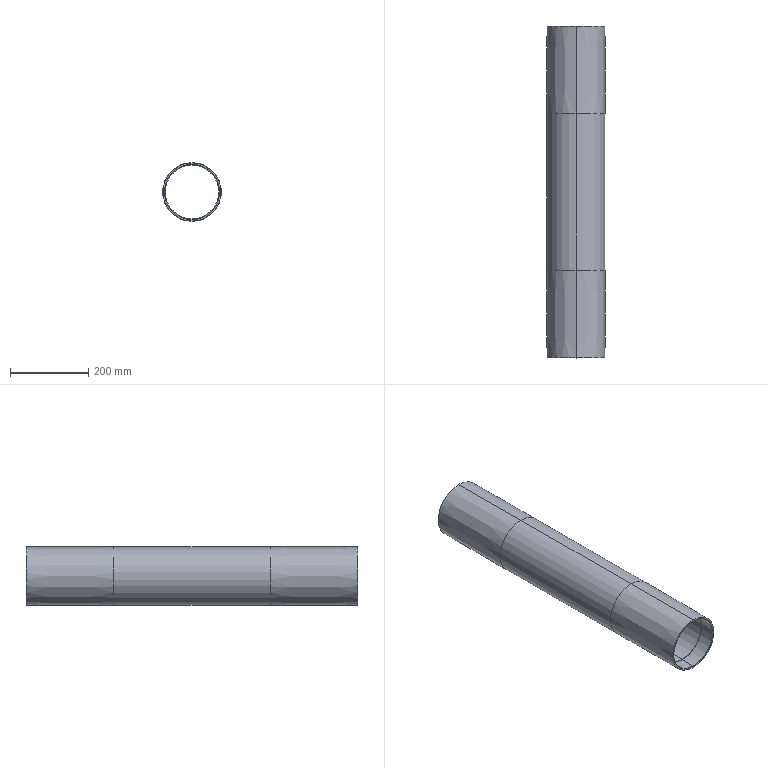Part | SolidWorks | features ICE 3, Chamfer 1, Revolution 1 | 1 solid | 20 faces | box 150 x 850 x 150 mm | volume 2218913 mm3 | cone 8 | cylinder 8 | plane 4 | commonest cylinder face diameters 140 x4 138 x2 150 x2
STEP:
#1=CARTESIAN_POINT('',(74.5,1.,70.));
#2=VERTEX_POINT('',#1);
#3=CARTESIAN_POINT('',(74.5,1.,-70.));
#4=VERTEX_POINT('',#3);
#5=CARTESIAN_POINT('',(74.5,1.,0.));
#6=DIRECTION('',(0.,-1.,0.));
#7=DIRECTION('',(0.,0.,-1.));
#8=AXIS2_PLACEMENT_3D('',#5,#6,#7);
#9=CIRCLE('',#8,70.);
#10=EDGE_CURVE('',#2,#4,#9,.T.);
#11=ORIENTED_EDGE('',*,*,#10,.F.);
#12=CARTESIAN_POINT('',(74.5,0.,71.));
#13=VERTEX_POINT('',#12);
#14=CARTESIAN_POINT('',(74.5,1.,70.));
#15=DIRECTION('',(0.,-0.7071,0.7071));
#16=VECTOR('',#15,1000.);
#17=LINE('',#14,#16);
#18=EDGE_CURVE('',#2,#13,#17,.T.);
#19=ORIENTED_EDGE('',*,*,#18,.T.);
#20=CARTESIAN_POINT('',(74.5,0.,-71.));
#21=VERTEX_POINT('',#20);
#22=CARTESIAN_POINT('',(74.5,0.,0.));
#23=DIRECTION('',(0.,1.,0.));
#24=DIRECTION('',(0.,0.,-1.));
#25=AXIS2_PLACEMENT_3D('',#22,#23,#24);
#26=CIRCLE('',#25,71.);
#27=EDGE_CURVE('',#21,#13,#26,.T.);
#28=ORIENTED_EDGE('',*,*,#27,.F.);
#29=CARTESIAN_POINT('',(74.5,1.,-70.));
#30=DIRECTION('',(0.,-0.7071,-0.7071));
#31=VECTOR('',#30,1000.);
#32=LINE('',#29,#31);
#33=EDGE_CURVE('',#4,#21,#32,.T.);
#34=ORIENTED_EDGE('',*,*,#33,.F.);
#35=EDGE_LOOP('',(#11,#19,#28,#34));
#36=FACE_OUTER_BOUND('',#35,.T.);
#37=CARTESIAN_POINT('',(74.5,1.,0.));
#38=DIRECTION('',(0.,-1.,0.));
#39=DIRECTION('',(0.,0.,-1.));
#40=AXIS2_PLACEMENT_3D('',#37,#38,#39);
#41=CONICAL_SURFACE('',#40,70.,0.7854);
#42=ADVANCED_FACE('',(#36),#41,.F.);
#43=CARTESIAN_POINT('',(74.5,849.,-70.));
#44=VERTEX_POINT('',#43);
#45=CARTESIAN_POINT('',(74.5,849.,70.));
#46=VERTEX_POINT('',#45);
#47=CARTESIAN_POINT('',(74.5,849.,0.));
#48=DIRECTION('',(0.,1.,0.));
#49=DIRECTION('',(0.,0.,1.));
#50=AXIS2_PLACEMENT_3D('',#47,#48,#49);
#51=CIRCLE('',#50,70.);
#52=EDGE_CURVE('',#44,#46,#51,.T.);
#53=ORIENTED_EDGE('',*,*,#52,.F.);
#54=CARTESIAN_POINT('',(74.5,850.,-71.));
#55=VERTEX_POINT('',#54);
#56=CARTESIAN_POINT('',(74.5,849.,-70.));
#57=DIRECTION('',(0.,0.7071,-0.7071));
#58=VECTOR('',#57,1000.);
#59=LINE('',#56,#58);
#60=EDGE_CURVE('',#44,#55,#59,.T.);
#61=ORIENTED_EDGE('',*,*,#60,.T.);
#62=CARTESIAN_POINT('',(74.5,850.,71.));
#63=VERTEX_POINT('',#62);
#64=CARTESIAN_POINT('',(74.5,850.,0.));
#65=DIRECTION('',(0.,-1.,0.));
#66=DIRECTION('',(0.,0.,1.));
#67=AXIS2_PLACEMENT_3D('',#64,#65,#66);
#68=CIRCLE('',#67,71.);
#69=EDGE_CURVE('',#63,#55,#68,.T.);
#70=ORIENTED_EDGE('',*,*,#69,.F.);
#71=CARTESIAN_POINT('',(74.5,849.,70.));
#72=DIRECTION('',(0.,0.7071,0.7071));
#73=VECTOR('',#72,1000.);
#74=LINE('',#71,#73);
#75=EDGE_CURVE('',#46,#63,#74,.T.);
#76=ORIENTED_EDGE('',*,*,#75,.F.);
#77=EDGE_LOOP('',(#53,#61,#70,#76));
#78=FACE_OUTER_BOUND('',#77,.T.);
#79=CARTESIAN_POINT('',(74.5,849.,0.));
#80=DIRECTION('',(0.,1.,0.));
#81=DIRECTION('',(0.,0.,1.));
#82=AXIS2_PLACEMENT_3D('',#79,#80,#81);
#83=CONICAL_SURFACE('',#82,70.,0.7854);
#84=ADVANCED_FACE('',(#78),#83,.F.);
#85=CARTESIAN_POINT('',(74.5,810.,-69.));
#86=VERTEX_POINT('',#85);
#87=CARTESIAN_POINT('',(74.5,810.,69.));
#88=VERTEX_POINT('',#87);
#89=CARTESIAN_POINT('',(74.5,810.,0.));
#90=DIRECTION('',(0.,1.,0.));
#91=DIRECTION('',(0.,0.,1.));
#92=AXIS2_PLACEMENT_3D('',#89,#90,#91);
#93=CIRCLE('',#92,69.);
#94=EDGE_CURVE('',#86,#88,#93,.T.);
#95=ORIENTED_EDGE('',*,*,#94,.T.);
#96=CARTESIAN_POINT('',(74.5,40.,69.));
#97=VERTEX_POINT('',#96);
#98=CARTESIAN_POINT('',(74.5,883.,69.));
#99=DIRECTION('',(0.,-1.,0.));
#100=VECTOR('',#99,1000.);
#101=LINE('',#98,#100);
#102=EDGE_CURVE('',#88,#97,#101,.T.);
#103=ORIENTED_EDGE('',*,*,#102,.T.);
#104=CARTESIAN_POINT('',(74.5,40.,-69.));
#105=VERTEX_POINT('',#104);
#106=CARTESIAN_POINT('',(74.5,40.,0.));
#107=DIRECTION('',(0.,-1.,0.));
#108=DIRECTION('',(0.,0.,-1.));
#109=AXIS2_PLACEMENT_3D('',#106,#107,#108);
#110=CIRCLE('',#109,69.);
#111=EDGE_CURVE('',#97,#105,#110,.T.);
#112=ORIENTED_EDGE('',*,*,#111,.T.);
#113=CARTESIAN_POINT('',(74.5,883.,-69.));
#114=DIRECTION('',(0.,-1.,0.));
#115=VECTOR('',#114,1000.);
#116=LINE('',#113,#115);
#117=EDGE_CURVE('',#86,#105,#116,.T.);
#118=ORIENTED_EDGE('',*,*,#117,.F.);
#119=EDGE_LOOP('',(#95,#103,#112,#118));
#120=FACE_OUTER_BOUND('',#119,.T.);
#121=CARTESIAN_POINT('',(74.5,883.,0.));
#122=DIRECTION('',(0.,-1.,0.));
#123=DIRECTION('',(0.,0.,-1.));
#124=AXIS2_PLACEMENT_3D('',#121,#122,#123);
#125=CYLINDRICAL_SURFACE('',#124,69.);
#126=ADVANCED_FACE('',(#120),#125,.F.);
#127=CARTESIAN_POINT('',(74.5,40.,70.));
#128=VERTEX_POINT('',#127);
#129=CARTESIAN_POINT('',(74.5,40.,-70.));
#130=VERTEX_POINT('',#129);
#131=CARTESIAN_POINT('',(74.5,40.,0.));
#132=DIRECTION('',(0.,-1.,0.));
#133=DIRECTION('',(0.,0.,-1.));
#134=AXIS2_PLACEMENT_3D('',#131,#132,#133);
#135=CIRCLE('',#134,70.);
#136=EDGE_CURVE('',#128,#130,#135,.T.);
#137=ORIENTED_EDGE('',*,*,#136,.F.);
#138=CARTESIAN_POINT('',(74.5,40.,70.));
#139=DIRECTION('',(0.,-1.,0.));
#140=VECTOR('',#139,1000.);
#141=LINE('',#138,#140);
#142=EDGE_CURVE('',#128,#2,#141,.T.);
#143=ORIENTED_EDGE('',*,*,#142,.T.);
#144=ORIENTED_EDGE('',*,*,#10,.T.);
#145=CARTESIAN_POINT('',(74.5,40.,-70.));
#146=DIRECTION('',(0.,-1.,0.));
#147=VECTOR('',#146,1000.);
#148=LINE('',#145,#147);
#149=EDGE_CURVE('',#130,#4,#148,.T.);
#150=ORIENTED_EDGE('',*,*,#149,.F.);
#151=EDGE_LOOP('',(#137,#143,#144,#150));
#152=FACE_OUTER_BOUND('',#151,.T.);
#153=CARTESIAN_POINT('',(74.5,40.,0.));
#154=DIRECTION('',(0.,-1.,0.));
#155=DIRECTION('',(0.,0.,-1.));
#156=AXIS2_PLACEMENT_3D('',#153,#154,#155);
#157=CYLINDRICAL_SURFACE('',#156,70.);
#158=ADVANCED_FACE('',(#152),#157,.F.);
#159=CARTESIAN_POINT('',(74.5,810.,-70.));
#160=VERTEX_POINT('',#159);
#161=CARTESIAN_POINT('',(74.5,810.,70.));
#162=VERTEX_POINT('',#161);
#163=CARTESIAN_POINT('',(74.5,810.,0.));
#164=DIRECTION('',(0.,1.,0.));
#165=DIRECTION('',(0.,0.,1.));
#166=AXIS2_PLACEMENT_3D('',#163,#164,#165);
#167=CIRCLE('',#166,70.);
#168=EDGE_CURVE('',#160,#162,#167,.T.);
#169=ORIENTED_EDGE('',*,*,#168,.F.);
#170=CARTESIAN_POINT('',(74.5,810.,-70.));
#171=DIRECTION('',(0.,1.,0.));
#172=VECTOR('',#171,1000.);
#173=LINE('',#170,#172);
#174=EDGE_CURVE('',#160,#44,#173,.T.);
#175=ORIENTED_EDGE('',*,*,#174,.T.);
#176=ORIENTED_EDGE('',*,*,#52,.T.);
#177=CARTESIAN_POINT('',(74.5,810.,70.));
#178=DIRECTION('',(0.,1.,0.));
#179=VECTOR('',#178,1000.);
#180=LINE('',#177,#179);
#181=EDGE_CURVE('',#162,#46,#180,.T.);
#182=ORIENTED_EDGE('',*,*,#181,.F.);
#183=EDGE_LOOP('',(#169,#175,#176,#182));
#184=FACE_OUTER_BOUND('',#183,.T.);
#185=CARTESIAN_POINT('',(74.5,810.,0.));
#186=DIRECTION('',(0.,1.,0.));
#187=DIRECTION('',(0.,0.,1.));
#188=AXIS2_PLACEMENT_3D('',#185,#186,#187);
#189=CYLINDRICAL_SURFACE('',#188,70.);
#190=ADVANCED_FACE('',(#184),#189,.F.);
#191=CARTESIAN_POINT('',(74.5,0.,74.5));
#192=VERTEX_POINT('',#191);
#193=CARTESIAN_POINT('',(74.5,0.,-74.5));
#194=VERTEX_POINT('',#193);
#195=CARTESIAN_POINT('',(74.5,0.,0.));
#196=DIRECTION('',(0.,1.,0.));
#197=DIRECTION('',(0.,0.,1.));
#198=AXIS2_PLACEMENT_3D('',#195,#196,#197);
#199=CIRCLE('',#198,74.5);
#200=EDGE_CURVE('',#192,#194,#199,.T.);
#201=ORIENTED_EDGE('',*,*,#200,.T.);
#202=CARTESIAN_POINT('',(74.5,225.,-75.));
#203=VERTEX_POINT('',#202);
#204=CARTESIAN_POINT('',(74.5,225.,-75.));
#205=DIRECTION('',(0.,1.,-0.002222));
#206=VECTOR('',#205,1000.);
#207=LINE('',#204,#206);
#208=EDGE_CURVE('',#194,#203,#207,.T.);
#209=ORIENTED_EDGE('',*,*,#208,.T.);
#210=CARTESIAN_POINT('',(74.5,225.,75.));
#211=VERTEX_POINT('',#210);
#212=CARTESIAN_POINT('',(74.5,225.,0.));
#213=DIRECTION('',(0.,1.,0.));
#214=DIRECTION('',(0.,0.,1.));
#215=AXIS2_PLACEMENT_3D('',#212,#213,#214);
#216=CIRCLE('',#215,75.);
#217=EDGE_CURVE('',#211,#203,#216,.T.);
#218=ORIENTED_EDGE('',*,*,#217,.F.);
#219=CARTESIAN_POINT('',(74.5,225.,75.));
#220=DIRECTION('',(0.,1.,0.002222));
#221=VECTOR('',#220,1000.);
#222=LINE('',#219,#221);
#223=EDGE_CURVE('',#192,#211,#222,.T.);
#224=ORIENTED_EDGE('',*,*,#223,.F.);
#225=EDGE_LOOP('',(#201,#209,#218,#224));
#226=FACE_OUTER_BOUND('',#225,.T.);
#227=CARTESIAN_POINT('',(74.5,225.,0.));
#228=DIRECTION('',(0.,1.,0.));
#229=DIRECTION('',(0.,0.,1.));
#230=AXIS2_PLACEMENT_3D('',#227,#228,#229);
#231=CONICAL_SURFACE('',#230,75.,0.002222);
#232=ADVANCED_FACE('',(#226),#231,.T.);
#233=ORIENTED_EDGE('',*,*,#217,.T.);
#234=CARTESIAN_POINT('',(74.5,625.,-75.));
#235=VERTEX_POINT('',#234);
#236=CARTESIAN_POINT('',(74.5,850.,-75.));
#237=DIRECTION('',(0.,1.,0.));
#238=VECTOR('',#237,1000.);
#239=LINE('',#236,#238);
#240=EDGE_CURVE('',#203,#235,#239,.T.);
#241=ORIENTED_EDGE('',*,*,#240,.T.);
#242=CARTESIAN_POINT('',(74.5,625.,75.));
#243=VERTEX_POINT('',#242);
#244=CARTESIAN_POINT('',(74.5,625.,0.));
#245=DIRECTION('',(0.,1.,0.));
#246=DIRECTION('',(0.,0.,1.));
#247=AXIS2_PLACEMENT_3D('',#244,#245,#246);
#248=CIRCLE('',#247,75.);
#249=EDGE_CURVE('',#243,#235,#248,.T.);
#250=ORIENTED_EDGE('',*,*,#249,.F.);
#251=CARTESIAN_POINT('',(74.5,850.,75.));
#252=DIRECTION('',(0.,1.,0.));
#253=VECTOR('',#252,1000.);
#254=LINE('',#251,#253);
#255=EDGE_CURVE('',#211,#243,#254,.T.);
#256=ORIENTED_EDGE('',*,*,#255,.F.);
#257=EDGE_LOOP('',(#233,#241,#250,#256));
#258=FACE_OUTER_BOUND('',#257,.T.);
#259=CARTESIAN_POINT('',(74.5,850.,0.));
#260=DIRECTION('',(0.,1.,0.));
#261=DIRECTION('',(0.,0.,1.));
#262=AXIS2_PLACEMENT_3D('',#259,#260,#261);
#263=CYLINDRICAL_SURFACE('',#262,75.);
#264=ADVANCED_FACE('',(#258),#263,.T.);
#265=CARTESIAN_POINT('',(74.5,850.,74.5));
#266=VERTEX_POINT('',#265);
#267=CARTESIAN_POINT('',(74.5,850.,-74.5));
#268=VERTEX_POINT('',#267);
#269=CARTESIAN_POINT('',(74.5,850.,0.));
#270=DIRECTION('',(0.,1.,0.));
#271=DIRECTION('',(0.,0.,1.));
#272=AXIS2_PLACEMENT_3D('',#269,#270,#271);
#273=CIRCLE('',#272,74.5);
#274=EDGE_CURVE('',#266,#268,#273,.T.);
#275=ORIENTED_EDGE('',*,*,#274,.F.);
#276=CARTESIAN_POINT('',(74.5,850.,74.5));
#277=DIRECTION('',(0.,-1.,0.002222));
#278=VECTOR('',#277,1000.);
#279=LINE('',#276,#278);
#280=EDGE_CURVE('',#266,#243,#279,.T.);
#281=ORIENTED_EDGE('',*,*,#280,.T.);
#282=ORIENTED_EDGE('',*,*,#249,.T.);
#283=CARTESIAN_POINT('',(74.5,850.,-74.5));
#284=DIRECTION('',(0.,-1.,-0.002222));
#285=VECTOR('',#284,1000.);
#286=LINE('',#283,#285);
#287=EDGE_CURVE('',#268,#235,#286,.T.);
#288=ORIENTED_EDGE('',*,*,#287,.F.);
#289=EDGE_LOOP('',(#275,#281,#282,#288));
#290=FACE_OUTER_BOUND('',#289,.T.);
#291=CARTESIAN_POINT('',(74.5,850.,0.));
#292=DIRECTION('',(0.,-1.,0.));
#293=DIRECTION('',(0.,0.,-1.));
#294=AXIS2_PLACEMENT_3D('',#291,#292,#293);
#295=CONICAL_SURFACE('',#294,74.5,0.002222);
#296=ADVANCED_FACE('',(#290),#295,.T.);
#297=ORIENTED_EDGE('',*,*,#27,.T.);
#298=CARTESIAN_POINT('',(74.5,0.,0.));
#299=DIRECTION('',(0.,1.,0.));
#300=DIRECTION('',(0.,0.,-1.));
#301=AXIS2_PLACEMENT_3D('',#298,#299,#300);
#302=CIRCLE('',#301,71.);
#303=EDGE_CURVE('',#13,#21,#302,.T.);
#304=ORIENTED_EDGE('',*,*,#303,.T.);
#305=EDGE_LOOP('',(#297,#304));
#306=FACE_BOUND('',#305,.T.);
#307=ORIENTED_EDGE('',*,*,#200,.F.);
#308=CARTESIAN_POINT('',(74.5,0.,0.));
#309=DIRECTION('',(0.,1.,0.));
#310=DIRECTION('',(0.,0.,1.));
#311=AXIS2_PLACEMENT_3D('',#308,#309,#310);
#312=CIRCLE('',#311,74.5);
#313=EDGE_CURVE('',#194,#192,#312,.T.);
#314=ORIENTED_EDGE('',*,*,#313,.F.);
#315=EDGE_LOOP('',(#307,#314));
#316=FACE_OUTER_BOUND('',#315,.T.);
#317=CARTESIAN_POINT('',(0.,0.,0.));
#318=DIRECTION('',(0.,-1.,0.));
#319=DIRECTION('',(0.,0.,-1.));
#320=AXIS2_PLACEMENT_3D('',#317,#318,#319);
#321=PLANE('',#320);
#322=ADVANCED_FACE('',(#306,#316),#321,.T.);
#323=ORIENTED_EDGE('',*,*,#69,.T.);
#324=CARTESIAN_POINT('',(74.5,850.,0.));
#325=DIRECTION('',(0.,-1.,0.));
#326=DIRECTION('',(0.,0.,1.));
#327=AXIS2_PLACEMENT_3D('',#324,#325,#326);
#328=CIRCLE('',#327,71.);
#329=EDGE_CURVE('',#55,#63,#328,.T.);
#330=ORIENTED_EDGE('',*,*,#329,.T.);
#331=EDGE_LOOP('',(#323,#330));
#332=FACE_BOUND('',#331,.T.);
#333=CARTESIAN_POINT('',(74.5,850.,0.));
#334=DIRECTION('',(0.,1.,0.));
#335=DIRECTION('',(0.,0.,1.));
#336=AXIS2_PLACEMENT_3D('',#333,#334,#335);
#337=CIRCLE('',#336,74.5);
#338=EDGE_CURVE('',#268,#266,#337,.T.);
#339=ORIENTED_EDGE('',*,*,#338,.T.);
#340=ORIENTED_EDGE('',*,*,#274,.T.);
#341=EDGE_LOOP('',(#339,#340));
#342=FACE_OUTER_BOUND('',#341,.T.);
#343=CARTESIAN_POINT('',(0.,850.,0.));
#344=DIRECTION('',(0.,1.,0.));
#345=DIRECTION('',(0.,0.,1.));
#346=AXIS2_PLACEMENT_3D('',#343,#344,#345);
#347=PLANE('',#346);
#348=ADVANCED_FACE('',(#332,#342),#347,.T.);
#349=ORIENTED_EDGE('',*,*,#280,.F.);
#350=ORIENTED_EDGE('',*,*,#338,.F.);
#351=ORIENTED_EDGE('',*,*,#287,.T.);
#352=CARTESIAN_POINT('',(74.5,625.,0.));
#353=DIRECTION('',(0.,1.,0.));
#354=DIRECTION('',(0.,0.,1.));
#355=AXIS2_PLACEMENT_3D('',#352,#353,#354);
#356=CIRCLE('',#355,75.);
#357=EDGE_CURVE('',#235,#243,#356,.T.);
#358=ORIENTED_EDGE('',*,*,#357,.T.);
#359=EDGE_LOOP('',(#349,#350,#351,#358));
#360=FACE_OUTER_BOUND('',#359,.T.);
#361=CARTESIAN_POINT('',(74.5,850.,0.));
#362=DIRECTION('',(0.,-1.,0.));
#363=DIRECTION('',(0.,0.,-1.));
#364=AXIS2_PLACEMENT_3D('',#361,#362,#363);
#365=CONICAL_SURFACE('',#364,74.5,0.002222);
#366=ADVANCED_FACE('',(#360),#365,.T.);
#367=ORIENTED_EDGE('',*,*,#240,.F.);
#368=CARTESIAN_POINT('',(74.5,225.,0.));
#369=DIRECTION('',(0.,1.,0.));
#370=DIRECTION('',(0.,0.,1.));
#371=AXIS2_PLACEMENT_3D('',#368,#369,#370);
#372=CIRCLE('',#371,75.);
#373=EDGE_CURVE('',#203,#211,#372,.T.);
#374=ORIENTED_EDGE('',*,*,#373,.T.);
#375=ORIENTED_EDGE('',*,*,#255,.T.);
#376=ORIENTED_EDGE('',*,*,#357,.F.);
#377=EDGE_LOOP('',(#367,#374,#375,#376));
#378=FACE_OUTER_BOUND('',#377,.T.);
#379=CARTESIAN_POINT('',(74.5,850.,0.));
#380=DIRECTION('',(0.,1.,0.));
#381=DIRECTION('',(0.,0.,1.));
#382=AXIS2_PLACEMENT_3D('',#379,#380,#381);
#383=CYLINDRICAL_SURFACE('',#382,75.);
#384=ADVANCED_FACE('',(#378),#383,.T.);
#385=ORIENTED_EDGE('',*,*,#208,.F.);
#386=ORIENTED_EDGE('',*,*,#313,.T.);
#387=ORIENTED_EDGE('',*,*,#223,.T.);
#388=ORIENTED_EDGE('',*,*,#373,.F.);
#389=EDGE_LOOP('',(#385,#386,#387,#388));
#390=FACE_OUTER_BOUND('',#389,.T.);
#391=CARTESIAN_POINT('',(74.5,225.,0.));
#392=DIRECTION('',(0.,1.,0.));
#393=DIRECTION('',(0.,0.,1.));
#394=AXIS2_PLACEMENT_3D('',#391,#392,#393);
#395=CONICAL_SURFACE('',#394,75.,0.002222);
#396=ADVANCED_FACE('',(#390),#395,.T.);
#397=ORIENTED_EDGE('',*,*,#174,.F.);
#398=CARTESIAN_POINT('',(74.5,810.,0.));
#399=DIRECTION('',(0.,1.,0.));
#400=DIRECTION('',(0.,0.,1.));
#401=AXIS2_PLACEMENT_3D('',#398,#399,#400);
#402=CIRCLE('',#401,70.);
#403=EDGE_CURVE('',#162,#160,#402,.T.);
#404=ORIENTED_EDGE('',*,*,#403,.F.);
#405=ORIENTED_EDGE('',*,*,#181,.T.);
#406=CARTESIAN_POINT('',(74.5,849.,0.));
#407=DIRECTION('',(0.,1.,0.));
#408=DIRECTION('',(0.,0.,1.));
#409=AXIS2_PLACEMENT_3D('',#406,#407,#408);
#410=CIRCLE('',#409,70.);
#411=EDGE_CURVE('',#46,#44,#410,.T.);
#412=ORIENTED_EDGE('',*,*,#411,.T.);
#413=EDGE_LOOP('',(#397,#404,#405,#412));
#414=FACE_OUTER_BOUND('',#413,.T.);
#415=CARTESIAN_POINT('',(74.5,810.,0.));
#416=DIRECTION('',(0.,1.,0.));
#417=DIRECTION('',(0.,0.,1.));
#418=AXIS2_PLACEMENT_3D('',#415,#416,#417);
#419=CYLINDRICAL_SURFACE('',#418,70.);
#420=ADVANCED_FACE('',(#414),#419,.F.);
#421=ORIENTED_EDGE('',*,*,#94,.F.);
#422=CARTESIAN_POINT('',(74.5,810.,0.));
#423=DIRECTION('',(0.,1.,0.));
#424=DIRECTION('',(0.,0.,1.));
#425=AXIS2_PLACEMENT_3D('',#422,#423,#424);
#426=CIRCLE('',#425,69.);
#427=EDGE_CURVE('',#88,#86,#426,.T.);
#428=ORIENTED_EDGE('',*,*,#427,.F.);
#429=EDGE_LOOP('',(#421,#428));
#430=FACE_BOUND('',#429,.T.);
#431=ORIENTED_EDGE('',*,*,#403,.T.);
#432=ORIENTED_EDGE('',*,*,#168,.T.);
#433=EDGE_LOOP('',(#431,#432));
#434=FACE_OUTER_BOUND('',#433,.T.);
#435=CARTESIAN_POINT('',(74.5,810.,0.));
#436=DIRECTION('',(0.,1.,0.));
#437=DIRECTION('',(0.,0.,1.));
#438=AXIS2_PLACEMENT_3D('',#435,#436,#437);
#439=PLANE('',#438);
#440=ADVANCED_FACE('',(#430,#434),#439,.T.);
#441=ORIENTED_EDGE('',*,*,#142,.F.);
#442=CARTESIAN_POINT('',(74.5,40.,0.));
#443=DIRECTION('',(0.,-1.,0.));
#444=DIRECTION('',(0.,0.,-1.));
#445=AXIS2_PLACEMENT_3D('',#442,#443,#444);
#446=CIRCLE('',#445,70.);
#447=EDGE_CURVE('',#130,#128,#446,.T.);
#448=ORIENTED_EDGE('',*,*,#447,.F.);
#449=ORIENTED_EDGE('',*,*,#149,.T.);
#450=CARTESIAN_POINT('',(74.5,1.,0.));
#451=DIRECTION('',(0.,-1.,0.));
#452=DIRECTION('',(0.,0.,-1.));
#453=AXIS2_PLACEMENT_3D('',#450,#451,#452);
#454=CIRCLE('',#453,70.);
#455=EDGE_CURVE('',#4,#2,#454,.T.);
#456=ORIENTED_EDGE('',*,*,#455,.T.);
#457=EDGE_LOOP('',(#441,#448,#449,#456));
#458=FACE_OUTER_BOUND('',#457,.T.);
#459=CARTESIAN_POINT('',(74.5,40.,0.));
#460=DIRECTION('',(0.,-1.,0.));
#461=DIRECTION('',(0.,0.,-1.));
#462=AXIS2_PLACEMENT_3D('',#459,#460,#461);
#463=CYLINDRICAL_SURFACE('',#462,70.);
#464=ADVANCED_FACE('',(#458),#463,.F.);
#465=CARTESIAN_POINT('',(74.5,40.,0.));
#466=DIRECTION('',(0.,-1.,0.));
#467=DIRECTION('',(0.,0.,-1.));
#468=AXIS2_PLACEMENT_3D('',#465,#466,#467);
#469=CIRCLE('',#468,69.);
#470=EDGE_CURVE('',#105,#97,#469,.T.);
#471=ORIENTED_EDGE('',*,*,#470,.F.);
#472=ORIENTED_EDGE('',*,*,#111,.F.);
#473=EDGE_LOOP('',(#471,#472));
#474=FACE_BOUND('',#473,.T.);
#475=ORIENTED_EDGE('',*,*,#447,.T.);
#476=ORIENTED_EDGE('',*,*,#136,.T.);
#477=EDGE_LOOP('',(#475,#476));
#478=FACE_OUTER_BOUND('',#477,.T.);
#479=CARTESIAN_POINT('',(74.5,40.,0.));
#480=DIRECTION('',(0.,-1.,0.));
#481=DIRECTION('',(0.,0.,-1.));
#482=AXIS2_PLACEMENT_3D('',#479,#480,#481);
#483=PLANE('',#482);
#484=ADVANCED_FACE('',(#474,#478),#483,.T.);
#485=ORIENTED_EDGE('',*,*,#102,.F.);
#486=ORIENTED_EDGE('',*,*,#427,.T.);
#487=ORIENTED_EDGE('',*,*,#117,.T.);
#488=ORIENTED_EDGE('',*,*,#470,.T.);
#489=EDGE_LOOP('',(#485,#486,#487,#488));
#490=FACE_OUTER_BOUND('',#489,.T.);
#491=CARTESIAN_POINT('',(74.5,883.,0.));
#492=DIRECTION('',(0.,-1.,0.));
#493=DIRECTION('',(0.,0.,-1.));
#494=AXIS2_PLACEMENT_3D('',#491,#492,#493);
#495=CYLINDRICAL_SURFACE('',#494,69.);
#496=ADVANCED_FACE('',(#490),#495,.F.);
#497=ORIENTED_EDGE('',*,*,#60,.F.);
#498=ORIENTED_EDGE('',*,*,#411,.F.);
#499=ORIENTED_EDGE('',*,*,#75,.T.);
#500=ORIENTED_EDGE('',*,*,#329,.F.);
#501=EDGE_LOOP('',(#497,#498,#499,#500));
#502=FACE_OUTER_BOUND('',#501,.T.);
#503=CARTESIAN_POINT('',(74.5,849.,0.));
#504=DIRECTION('',(0.,1.,0.));
#505=DIRECTION('',(0.,0.,1.));
#506=AXIS2_PLACEMENT_3D('',#503,#504,#505);
#507=CONICAL_SURFACE('',#506,70.,0.7854);
#508=ADVANCED_FACE('',(#502),#507,.F.);
#509=ORIENTED_EDGE('',*,*,#18,.F.);
#510=ORIENTED_EDGE('',*,*,#455,.F.);
#511=ORIENTED_EDGE('',*,*,#33,.T.);
#512=ORIENTED_EDGE('',*,*,#303,.F.);
#513=EDGE_LOOP('',(#509,#510,#511,#512));
#514=FACE_OUTER_BOUND('',#513,.T.);
#515=CARTESIAN_POINT('',(74.5,1.,0.));
#516=DIRECTION('',(0.,-1.,0.));
#517=DIRECTION('',(0.,0.,-1.));
#518=AXIS2_PLACEMENT_3D('',#515,#516,#517);
#519=CONICAL_SURFACE('',#518,70.,0.7854);
#520=ADVANCED_FACE('',(#514),#519,.F.);
#521=CLOSED_SHELL('',(#42,#84,#126,#158,#190,#232,#264,#296,#322,#348,#366,#384,#396,#420,#440,#464,#484,#496,#508,#520));
#522=MANIFOLD_SOLID_BREP('',#521);
#523=CARTESIAN_POINT('',(0.,0.,0.));
#524=DIRECTION('',(0.,0.,1.));
#525=DIRECTION('',(1.,0.,0.));
#526=AXIS2_PLACEMENT_3D('',#523,#524,#525);
#527=(LENGTH_UNIT()NAMED_UNIT(*)SI_UNIT(.MILLI.,.METRE.));
#528=UNCERTAINTY_MEASURE_WITH_UNIT(LENGTH_MEASURE(0.00001),#527,'','');
#529=(NAMED_UNIT(*)PLANE_ANGLE_UNIT()SI_UNIT($,.RADIAN.));
#530=(NAMED_UNIT(*)SI_UNIT($,.STERADIAN.)SOLID_ANGLE_UNIT());
#531=(GEOMETRIC_REPRESENTATION_CONTEXT(3)GLOBAL_UNCERTAINTY_ASSIGNED_CONTEXT((#528))GLOBAL_UNIT_ASSIGNED_CONTEXT((#527,#529,#530))REPRESENTATION_CONTEXT('',''));
#532=ADVANCED_BREP_SHAPE_REPRESENTATION('',(#522,#526),#531);